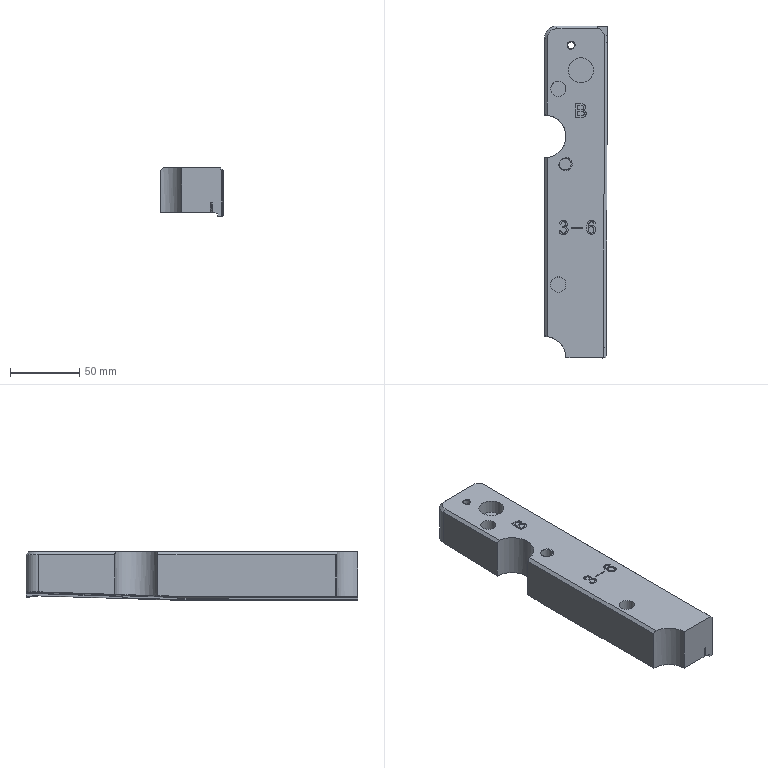NC program | NX | posted with a generic post | part box 45.476 x 239.737 x 35.001 mm
Lines 3829 to 4891 of 16758:
(CAVITY_MILL_2_COPY_COPY , TOOL : D16R0.8)
N7620 M6
N7622 G53
N7624 G17 G0 G90 X0.001 Y34.455 S2500 M3
N7626 G43 Z60. H0
N7628 G94 G1 Z35.502 F4000.
N7630 Z35.302 F1380.
N7632 Y23.255
N7634 X119.894 F2300.
N7636 G2 X120.382 Y22.789 R0.488
N7638 G1 X120.384 Y22.67
N7640 X120.387 Y-22.681
N7642 X120.385 Y-22.757
N7644 G2 X119.873 Y-23.255 R0.512
N7646 G1 X-119.865
N7648 G2 X-120.384 Y-22.735 R0.52
N7650 G1 X-120.383 Y22.748
N7652 G2 X-119.876 Y23.255 R0.507
N7654 G1 X0.001
N7656 Y13.895
N7658 X111.025
N7660 X111.027 Y-13.895
N7662 X-111.024
N7664 Y13.895
N7666 X0.001
N7668 Y4.535
N7670 X101.665
N7672 X101.666 Y-4.535
N7674 X-101.664
N7676 Y4.535
N7678 X0.001
N7680 Y15.735
N7682 Z35.502
N7684 G0 Z36.501
N7686 X0. Y34.626
N7688 G1 Z35.303 F4000.
N7690 Z35.103 F1380.
N7692 Y23.426
N7694 X119.382 F2300.
N7696 X120.095 Y23.387
N7698 G2 X120.557 Y22.846 R0.71
N7700 G1 X120.556 Y-22.731
N7702 G2 X119.86 Y-23.426 R0.695
N7704 G1 X-119.856
N7706 G2 X-120.557 Y-22.726 R0.7
N7708 G1 X-120.556 Y22.727
N7710 G2 X-119.857 Y23.426 R0.699
N7712 G1 X0.
N7714 Y14.066
N7716 X111.196
N7718 Y-14.066
N7720 X-111.197
N7722 X-111.196 Y14.066
N7724 X0.
N7726 Y4.706
N7728 X101.836
N7730 Y-4.706
N7732 X-101.836
N7734 Y4.706
N7736 X0.
N7738 Y15.906
N7740 Z35.303
N7742 G0 Z36.302
N7744 Y-34.698
N7746 G1 Z35.104 F4000.
N7748 Z34.904 F1380.
N7750 Y-23.498
N7752 X-119.893 F2300.
N7754 G2 X-120.628 Y-22.763 R0.735
N7756 G1 Y9.225
N7758 G2 X-127.828 Y13.401 R9.78
N7760 G1 Y22.763
N7762 G2 X-119.892 Y30.698 R7.935
N7764 G1 X18.758
N7766 G2 X24.095 Y23.498 R9.198
N7768 G1 X119.871
N7770 G2 X120.626 Y22.786 R0.757
N7772 G1 X120.628 Y22.753
N7774 Y-22.744
N7776 G2 X119.874 Y-23.498 R0.754
N7778 G1 X0.
N7780 Y-14.138
N7782 X-111.268
N7784 Y9.225
N7786 Y9.236
N7788 X-31.236 Y9.681
N7790 X-31.159 Y9.68
N7792 X-30.139 Y9.685
N7794 X-30.126
N7796 X10.322 Y10.191
N7798 G3 X10.94 Y10.218 R9.834
N7800 G1 X11.005 Y10.224
N7802 X15.047 Y10.672
N7804 X15.182 Y10.692
N7806 X16.595 Y10.954
N7808 G3 X22.188 Y14.334 R9.266
N7810 G1 X20.717 Y15.492
N7812 G2 X16.254 Y12.794 R7.394
N7814 G1 X14.841 Y12.532
N7816 X10.799 Y12.085
N7818 G2 X10.299 Y12.063 R7.962
N7820 G1 X-30.15 Y11.557
N7822 X-31.169 Y11.552
N7824 X-31.176 Y11.553
N7826 X-119.826 Y11.061
N7828 G2 X-127.695 Y19.051 R7.908
N7830 G1 Y21.655
N7832 G2 X-119.907 Y29.486 R7.877
N7834 G1 X-112.141 Y29.53
N7836 X10.126 Y30.106
N7838 G2 X16.365 Y29.507 R32.892
N7840 X22.3 Y22.314 R7.326
N7842 G1 Y20.064
N7844 G2 X20.717 Y15.492 R7.394
N7846 G1 X22.188 Y14.334
N7848 G3 X24.095 Y14.138 R9.36
N7850 G1 X111.268
N7852 Y-14.138
N7854 X0.
N7856 Y-4.778
N7858 X-101.908
N7860 Y-0.072
N7862 X-31.281 Y0.32
N7864 X-31.204 Y0.319
N7866 X-30.071 Y0.326
N7868 X-30.025
N7870 X10.439 Y0.832
N7872 G3 X11.727 Y0.891 R19.194
N7874 G1 X11.954 Y0.912
N7876 X16.077 Y1.369
N7878 G3 X16.888 Y1.489 R11.232
N7880 G1 X18.301 Y1.751
N7882 G3 X25.548 Y4.778 R18.626
N7884 G1 X101.908
N7886 Y-4.778
N7888 X0.
N7890 Y-15.978
N7892 Z35.104
N7894 G0 Z36.103
N7896 X65.496 Y-34.737
N7898 G1 Z34.905 F4000.
N7900 Z34.705 F1380.
N7902 Y-23.537
N7904 X-119.857 F2300.
N7906 G2 X-120.668 Y-22.726 R0.811
N7908 G1 Y8.941
N7910 G2 X-127.868 Y13.053 R10.045
N7912 G1 Y18.186
N7914 G3 X-119.825 Y10.769 R8.173
N7916 G1 X-31.237 Y11.262
N7918 X-31.168 Y11.261
N7920 X-30.174 Y11.267
N7922 X-30.119
N7924 X10.302 Y11.772
N7926 G3 X10.582 Y11.781 R8.253
N7928 G1 X15.201 Y12.084
N7930 X19.819 Y12.387
N7932 X22.493 Y12.825
N7934 G3 X28.719 Y20.152 R7.425
N7936 G1 Y22.331
N7938 G3 X21.74 Y29.771 R7.546
N7940 X10.158 Y30.313 R138.168
N7942 G1 X-112.142 Y29.737
N7944 X-112.172 Y29.733
N7946 X-119.866 Y29.692
N7948 G3 X-127.868 Y22.394 R8.04
N7950 G1 Y22.728
N7952 G2 X-119.859 Y30.737 R8.009
N7954 G1 X25.248
N7956 G2 X30.503 Y23.537 R9.418
N7958 G1 X119.858
N7960 G2 X120.668 Y22.728 R0.809
N7962 G1 Y-22.726
N7964 G2 X119.857 Y-23.537 R0.811
N7966 G1 X65.496
N7968 Y-14.177
N7970 X-111.308
N7972 Y1.457
N7974 X-31.245 Y1.901
N7976 X-31.176
N7978 X-30.106 Y1.907
N7980 X-30.019 Y1.908
N7982 X10.419 Y2.413
N7984 G3 X11.106 Y2.435 R17.613
N7986 G1 X20.884 Y3.077
N7988 X24.004 Y3.588
N7990 G3 X36.98 Y14.177 R16.785
N7992 G1 X111.308
N7994 Y-14.177
N7996 X65.496
N7998 Y-4.817
N8000 X29.045
N8002 X21.886 Y-4.053
N8004 G2 X21.356 Y-4.108 R7.2
N8006 G1 X11.578 Y-4.75
N8008 X11.474 Y-4.756
N8010 G2 X10.509 Y-4.786 R24.813
N8012 G1 X-29.929 Y-5.292
N8014 X-29.954
N8016 X-30.041 Y-5.293
N8018 X-30.066
N8020 X-31.136 Y-5.299
N8022 X-31.229
N8024 X-31.252
N8026 X-104.108 Y-5.703
N8028 Y-6.977
N8030 X22.177
N8032 G2 X21.886 Y-4.053 R7.2
N8034 G1 X29.045 Y-4.817
N8036 G3 X42.47 Y4.817 R26.145
N8038 G1 X101.948
N8040 Y-4.817
N8042 X65.496
N8044 Y-16.017
N8046 Z34.905
N8048 G0 Z35.904
N8050 X68.725 Y-34.738
N8052 G1 Z34.707 F4000.
N8054 Z34.507 F1380.
N8056 Y-23.538
N8058 X-119.857 F2300.
N8060 G2 X-120.668 Y-22.726 R0.811
N8062 G1 Y8.754
N8064 G2 X-127.868 Y12.772 R10.07
N8066 G1 Y17.387
N8068 G3 X-119.824 Y10.587 R8.198
N8070 G1 X-31.206 Y11.08
N8072 X-31.167 Y11.079
N8074 X-30.145 Y11.085
N8076 X9.799 Y11.584
N8078 X10.305 Y11.591
N8080 X10.307
N8082 X10.495 Y11.595
N8084 G3 X28.35 Y12.722 R243.063
N8086 X35.138 Y20.225 R7.54
N8088 G1 Y22.367
N8090 G3 X28.133 Y29.847 R7.496
N8092 X10.159 Y30.422 R268.337
N8094 G1 X-112.142 Y29.846
N8096 X-112.172 Y29.831
N8098 X-119.867 Y29.792
N8100 G3 X-127.849 Y23.271 R8.137
N8102 G2 X-119.855 Y30.737 R8.013
N8104 G1 X31.849
N8106 G2 X36.937 Y23.537 R9.368
N8108 G1 X119.858
N8110 G2 X120.668 Y22.728 R0.81
N8112 G1 Y-22.726
N8114 G2 X119.856 Y-23.538 R0.811
N8116 G1 X68.725
N8118 Y-14.178
N8120 X-111.308
N8122 Y1.275
N8124 X-31.225 Y1.72
N8126 X-31.187 Y1.719
N8128 X-30.061 Y1.725
N8130 X10.426 Y2.231
N8132 G3 X10.774 Y2.239 R17.795
N8134 X29.283 Y3.409 R252.423
N8136 X43.379 Y14.177 R16.9
N8138 G1 X111.308
N8140 Y-14.178
N8142 X68.725
N8144 Y-4.818
N8146 X35.503
N8148 X28.359 Y-3.914
N8150 G2 X10.984 Y-4.958 R259.623
N8152 X10.516 Y-4.968 R24.995
N8154 G1 X-29.971 Y-5.474
N8156 X-30.021
N8158 X-31.147 Y-5.481
N8160 X-31.238
N8162 X-104.108 Y-5.886
N8164 Y-6.978
N8166 X28.634
N8168 G2 X28.359 Y-3.914 R7.2
N8170 G1 X35.503 Y-4.818
N8172 G3 X48.863 Y4.817 R26.26
N8174 G1 X101.948
N8176 Y-4.818
N8178 X68.725
N8180 Y-16.018
N8182 Z34.707
N8184 G0 Z35.705
N8186 X71.638 Y-34.738
N8188 G1 Z34.508 F4000.
N8190 Z34.308 F1380.
N8192 Y-23.538
N8194 X-119.857 F2300.
N8196 G2 X-120.668 Y-22.726 R0.811
N8198 G1 Y8.627
N8200 G2 X-127.868 Y12.595 R10.071
N8202 G1 Y17.045
N8204 G3 X-119.824 Y10.464 R8.199
N8206 G1 X-31.206 Y10.956
N8208 X-31.167
N8210 X-30.144 Y10.962
N8212 X10.306 Y11.468
N8214 X10.434 Y11.47
N8216 X10.758 Y11.493
N8218 G3 X14.853 Y11.605 R512.62
N8220 X32.063 Y12.434 R512.62
N8222 X36.386 Y13.246 R18.276
N8224 X41.558 Y20.305 R7.404
N8226 G1 Y22.392
N8228 X38.802 Y28.145
N8230 G3 X34.912 Y29.739 R7.536
N8232 G1 X31.398 Y30.114
N8234 G3 X10.159 Y30.472 R579.431
N8236 G1 X-50.992 Y30.184
N8238 X-112.142 Y29.897
N8240 X-112.172 Y29.891
N8242 X-119.868 Y29.852
N8244 G3 X-127.814 Y23.651 R8.201
N8246 G2 X-119.855 Y30.737 R8.013
N8248 G1 X38.163
N8250 G2 X39.967 Y29.61 R9.408
N8252 X40.491 Y28.953 R1.872
N8254 G1 X43.084 Y23.537
N8256 X119.858
N8258 G2 X120.668 Y22.728 R0.81
N8260 G1 Y-22.726
N8262 G2 X119.856 Y-23.538 R0.811
N8264 G1 X71.638
N8266 Y-14.178
N8268 X-111.308
N8270 Y1.151
N8272 X-31.2 Y1.596
N8274 X-31.16
N8276 X11.196 Y2.141
N8278 G3 X15.146 Y2.249 R521.98
N8280 X32.67 Y3.094 R521.98
N8282 X39.207 Y4.321 R27.636
N8284 X49.758 Y14.177 R16.764
N8286 G1 X111.308
N8288 Y-14.178
N8290 X71.638
N8292 Y-4.818
N8294 X41.328
N8296 X34.174 Y-4.008
N8298 G2 X33.138 Y-4.091 R34.836
N8300 X15.371 Y-4.947 R529.18
N8302 X11.367 Y-5.057 R529.18
N8304 G1 X11.288 Y-5.059
N8306 X-31.068 Y-5.603
N8308 X-31.19 Y-5.604
N8310 X-31.195
N8312 X-104.108 Y-6.009
N8314 Y-6.978
N8316 X34.46
N8318 G2 X34.174 Y-4.008 R7.2
N8320 G1 X41.328 Y-4.818
N8322 G3 X42.029 Y-4.604 R36.996
N8324 X55.192 Y4.817 R26.124
N8326 G1 X101.948
N8328 Y-4.818
N8330 X71.638
N8332 Y-16.018
N8334 Z34.508
N8336 G0 Z35.507
N8338 X74.712 Y-34.738
N8340 G1 Z34.309 F4000.
N8342 Z34.109 F1380.
N8344 Y-23.538
N8346 X-119.857 F2300.
N8348 G2 X-120.668 Y-22.726 R0.811
N8350 G1 Y8.544
N8352 G2 X-127.868 Y12.486 R10.069
N8354 G1 Y16.865
N8356 G3 X-119.823 Y10.383 R8.197
N8358 G1 X-31.206 Y10.875
N8360 X-31.167
N8362 X-30.172 Y10.881
N8364 X-30.115
N8366 X-10.031 Y11.132
N8368 X10.307 Y11.386
N8370 X10.347 Y11.387
N8372 X10.386 Y11.388
N8374 G3 X37.61 Y12.442 R719.899
N8376 X42.479 Y13.224 R24.33
N8378 X47.977 Y20.38 R7.407
N8380 G1 Y22.432
N8382 Y22.433
N8384 G3 X41.723 Y29.697 R7.347
N8386 X35.459 Y30.25 R51.438
N8388 X13.134 Y30.493 R694.868
N8390 G1 X-112.17 Y29.903
N8392 X-112.175
N8394 X-119.913 Y29.862
N8396 G3 X-127.806 Y23.723 R8.2
N8398 G2 X-119.855 Y30.737 R8.013
N8400 G1 X44.63
N8402 G2 X49.782 Y23.537 R9.219
N8404 G1 X119.858
N8406 G2 X120.668 Y22.728 R0.81
N8408 G1 Y-22.726
N8410 G2 X119.856 Y-23.538 R0.811
N8412 G1 X74.712
N8414 Y-14.178
N8416 X-111.308
N8418 Y1.07
N8420 X-31.181 Y1.515
N8422 X-31.142
N8424 X-30.104 Y1.521
N8426 X-30.014 Y1.522
N8428 X10.579 Y2.03
N8430 G3 X38.149 Y3.097 R729.258
N8432 X44.892 Y4.18 R33.69
N8434 X56.148 Y14.177 R16.767
N8436 G1 X111.308
N8438 Y-14.178
N8440 X74.712
N8442 Y-4.818
N8444 X47.476
N8446 X40.329 Y-3.95
N8448 G2 X38.564 Y-4.091 R40.89
N8450 X10.721 Y-5.169 R736.458
N8452 G1 X10.669 Y-5.17
N8454 X-29.924 Y-5.678
N8456 X-29.949
N8458 X-30.039 Y-5.679
N8460 X-30.064
N8462 X-31.102 Y-5.685
N8464 X-31.144
N8466 X-31.162
N8468 X-104.108 Y-6.09
N8470 Y-6.978
N8472 X40.608
N8474 G2 X40.329 Y-3.95 R7.2
N8476 G1 X47.476 Y-4.818
N8478 G3 X61.556 Y4.817 R26.127
N8480 G1 X101.948
N8482 Y-4.818
N8484 X74.712
N8486 Y-16.018
N8488 Z34.309
N8490 G0 Z35.308
N8492 X77.911 Y-34.738
N8494 G1 Z34.11 F4000.
N8496 Z33.91 F1380.
N8498 Y-23.538
N8500 X-119.857 F2300.
N8502 G2 X-120.668 Y-22.726 R0.811
N8504 G1 Y8.496
N8506 G2 X-127.868 Y12.42 R10.079
N8508 G1 Y16.739
N8510 G3 X-119.823 Y10.335 R8.207
N8512 G1 X-31.206 Y10.828
N8514 X-31.167
N8516 X-30.171 Y10.833
N8518 X-30.115 Y10.834
N8520 X10.344 Y11.34
N8522 X18.783 Y11.511
N8524 G3 X46.539 Y12.74 R509.608
N8526 X54.396 Y20.455 R8.499
N8528 G1 Y22.468
N8530 G3 X48.156 Y29.719 R7.333
N8532 X41.334 Y30.31 R54.268
N8534 X19.553 Y30.523 R800.697
N8536 G1 X-112.17 Y29.903
N8538 X-112.175
N8540 X-119.913 Y29.862
N8542 X-119.931
N8544 G3 X-127.806 Y23.723 R8.2
N8546 G2 X-119.855 Y30.738 R8.013
N8548 G1 X51.106
N8550 G2 X56.206 Y23.538 R9.205
N8552 G1 X119.858
N8554 G2 X120.668 Y22.728 R0.81
N8556 G1 Y-22.73
N8558 G2 X119.86 Y-23.538 R0.807
N8560 G1 X77.911
N8562 Y-14.178
N8564 X-111.308
N8566 Y1.022
N8568 X-31.165 Y1.468
N8570 X-31.126
N8572 X-30.103 Y1.474
N8574 X-30.014
N8576 X10.497 Y1.981
N8578 X18.958 Y2.152
N8580 G3 X47.208 Y3.403 R518.968
N8582 X62.345 Y14.178 R17.859
N8584 G1 X111.308
N8586 Y-14.178
N8588 X77.911
N8590 Y-4.818
N8592 X53.874
N8594 X46.74 Y-3.848
N8596 G2 X19.092 Y-5.046 R526.168
N8598 G1 X10.643 Y-5.218
N8600 X10.587 Y-5.219
N8602 X-29.924 Y-5.725
N8604 X-29.949
N8606 X-30.038 Y-5.726
N8608 X-30.063
N8610 X-31.086 Y-5.732
N8612 X-31.103
N8614 X-31.133
N8616 X-104.108 Y-6.138
N8618 Y-6.978
N8620 X47.006
N8622 G2 X46.74 Y-3.848 R7.2
N8624 G1 X53.874 Y-4.818
N8626 G3 X67.656 Y4.818 R27.219
N8628 G1 X101.948
N8630 Y-4.818
N8632 X77.911
N8634 Y-16.018
N8636 Z34.11
N8638 G0 Z35.109
N8640 X81.127 Y-34.738
N8642 G1 Z33.911 F4000.
N8644 Z33.711 F1380.
N8646 Y-23.538
N8648 X-119.857 F2300.
N8650 G2 X-120.668 Y-22.726 R0.811
N8652 G1 Y8.478
N8654 G2 X-127.868 Y12.397 R10.08
N8656 G1 Y16.702
N8658 G3 X-119.823 Y10.318 R8.208
N8660 G1 X-112.117 Y10.361
N8662 X-112.074
N8664 X-30.171 Y10.816
N8666 X-30.114 Y10.817
N8668 X11.017 Y11.331
N8670 G3 X27.906 Y11.649 R1621.992
N8672 G1 X36.631 Y11.919
N8674 G3 X53.512 Y12.87 R334.668
N8676 X60.815 Y20.49 R7.957
N8678 G1 Y22.494
N8680 G3 X54.652 Y29.734 R7.335
N8682 X48.352 Y30.321 R46.943
N8684 X25.973 Y30.553 R741.905
N8686 G1 X-112.17 Y29.903
N8688 X-112.175
N8690 X-119.913 Y29.862
N8692 G3 X-127.806 Y23.723 R8.2
N8694 G2 X-119.855 Y30.738 R8.013
N8696 G1 X57.58
N8698 G2 X62.628 Y23.538 R9.207
N8700 G1 X119.858
N8702 G2 X120.668 Y22.728 R0.81
N8704 G1 Y-22.73
N8706 G2 X119.86 Y-23.538 R0.807
N8708 G1 X81.127
N8710 Y-14.178
N8712 X-111.308
N8714 Y1.006
N8716 X-30.103 Y1.457
N8718 X-30.014
N8720 X11.139 Y1.972
N8722 G3 X28.163 Y2.292 R1631.352
N8724 G1 X36.921 Y2.564
N8726 G3 X54.274 Y3.541 R344.028
N8728 X68.865 Y14.178 R17.317
N8730 G1 X111.308
N8732 Y-14.178
N8734 X81.127
N8736 Y-4.818
N8738 X60.307
N8740 X53.184 Y-3.768
N8742 G2 X37.145 Y-4.633 R351.228
N8744 G1 X28.386 Y-4.905
N8746 X28.336 Y-4.906
N8748 G2 X11.229 Y-5.228 R1638.552
N8750 G1 X-29.924 Y-5.742
N8752 X-29.949
N8754 X-30.038 Y-5.743
N8756 X-30.063
N8758 X-104.108 Y-6.155
N8760 Y-6.978
N8762 X53.439
N8764 G2 X53.184 Y-3.768 R7.2
N8766 G1 X60.307 Y-4.818
N8768 G3 X74.223 Y4.818 R26.677
N8770 G1 X101.948
N8772 Y-4.818
N8774 X81.127
N8776 Y-16.018
N8778 Z33.911
N8780 G0 Z34.91
N8782 X84.383 Y-34.738
N8784 G1 Z33.712 F4000.
N8786 Z33.512 F1380.
N8788 Y-23.538
N8790 X-119.857 F2300.
N8792 G2 X-120.668 Y-22.726 R0.811
N8794 G1 Y8.473
N8796 G2 X-127.868 Y12.392 R10.079
N8798 G1 Y16.697
N8800 G3 X-119.823 Y10.313 R8.207
N8802 G1 X-112.074 Y10.356
N8804 X-30.171 Y10.811
N8806 X-30.114 Y10.812
N8808 X17.436 Y11.406
N8810 G3 X39.481 Y11.873 R1308.21
N8812 G1 X40.467 Y11.908
N8814 X42.438 Y11.965
N8816 X56.237 Y12.59
N8818 X60.324 Y12.941
N8820 G3 X67.235 Y20.472 R7.558
N8822 G1 Y22.547
N8824 G3 X61.444 Y29.684 R7.293
N8826 X56.938 Y30.235 R26.497
N8828 X32.392 Y30.583 R563.158
N8830 G1 X-112.17 Y29.903
N8832 X-112.175
N8834 X-119.913 Y29.862
N8836 G3 X-127.806 Y23.723 R8.2
N8838 G2 X-119.855 Y30.738 R8.013
N8840 G1 X64.055
N8842 G2 X69.053 Y23.538 R9.165
N8844 G1 X119.858
N8846 G2 X120.668 Y22.728 R0.81
N8848 G1 Y-22.73
N8850 G2 X119.86 Y-23.538 R0.807
N8852 G1 X84.383
N8854 Y-14.178
N8856 X-111.308
N8858 Y1.
N8860 X-30.103 Y1.451
N8862 X-30.014 Y1.452
N8864 X17.555 Y2.047
N8866 G3 X39.787 Y2.518 R1317.57
N8868 G1 X40.769 Y2.553
N8870 X42.785 Y2.611
N8872 X56.85 Y3.248
N8874 X61.126 Y3.616
N8876 G3 X75.38 Y14.178 R16.918
N8878 G1 X111.308
N8880 Y-14.178
N8882 X84.383
N8884 Y-4.818
N8886 X66.818
N8888 X59.7 Y-3.733
N8890 X57.467 Y-3.925
N8892 G2 X57.176 Y-3.945 R7.2
N8894 G1 X43.11 Y-4.581
N8896 X42.992 Y-4.586
N8898 X41.001 Y-4.643
N8900 X40.045 Y-4.677
N8902 X40.001 Y-4.679
N8904 G2 X17.645 Y-5.153 R1324.77
N8906 G1 X-29.924 Y-5.747
N8908 X-29.949
N8910 X-30.038 Y-5.748
N8912 X-30.063
N8914 X-104.108 Y-6.16
N8916 Y-6.978
N8918 X59.949
N8920 G2 X59.7 Y-3.733 R7.2
N8922 G1 X66.818 Y-4.818
N8924 G3 X80.783 Y4.818 R26.278
N8926 G1 X101.948
N8928 Y-4.818
N8930 X84.383
N8932 Y-16.018
N8934 Z33.712
N8936 G0 Z34.711
N8938 X87.501 Y-34.738
N8940 G1 Z33.514 F4000.
N8942 Z33.314 F1380.
N8944 Y-23.538
N8946 X-119.857 F2300.
N8948 G2 X-120.668 Y-22.726 R0.811
N8950 G1 Y8.468
N8952 G2 X-127.868 Y12.387 R10.079
N8954 G1 Y16.693
N8956 G3 X-119.823 Y10.308 R8.207
N8958 G1 X-112.074 Y10.351
N8960 X-110.202 Y10.361
N8962 X-30.171 Y10.806
N8964 X-30.114 Y10.807
N8966 X22.726 Y11.467
N8968 G3 X50.295 Y12.093 R1258.898
N8970 G1 X50.323 Y12.098
N8972 X54.695 Y12.21
N8974 G3 X66.59 Y12.938 R167.491
N8976 X73.654 Y20.48 R7.823
N8978 G1 Y22.565
N8980 G3 X67.609 Y29.773 R7.321
N8982 G1 X66.093 Y30.041
N8984 X60.18 Y30.399
N8986 G3 X38.811 Y30.613 R651.504
N8988 G1 X-112.17 Y29.903
N8990 X-112.173
N8992 X-112.175
N8994 X-119.913 Y29.862
N8996 G3 X-127.806 Y23.723 R8.2
N8998 G2 X-119.855 Y30.738 R8.013
N9000 G1 X70.541
N9002 G2 X75.474 Y23.538 R9.193
N9004 G1 X119.858
N9006 G2 X120.668 Y22.728 R0.81
N9008 G1 Y-22.73
N9010 G2 X119.86 Y-23.538 R0.807
N9012 G1 X87.501
N9014 Y-14.178
N9016 X-111.308
N9018 Y0.995
N9020 X-30.014 Y1.447
N9022 X22.839 Y2.108
N9024 G3 X50.61 Y2.738 R1268.258
N9026 G1 X51.198 Y2.758
N9028 X54.934 Y2.853
N9030 G3 X67.494 Y3.622 R176.851
N9032 X81.722 Y14.178 R17.183
N9034 G1 X111.308
N9036 Y-14.178
N9038 X87.501
N9040 Y-4.818
N9042 X73.055
N9044 X65.935 Y-3.749
N9046 G2 X55.118 Y-4.344 R184.051
N9048 G1 X51.411 Y-4.439
N9050 X50.852 Y-4.458
N9052 G2 X22.929 Y-5.092 R1275.458
N9054 G1 X-29.924 Y-5.752
N9056 X-29.974 Y-5.753
N9058 X-104.108 Y-6.165
N9060 Y-6.978
N9062 X66.187
N9064 G2 X65.935 Y-3.749 R7.2
N9066 G1 X73.055 Y-4.818
N9068 G3 X87.083 Y4.818 R26.543
N9070 G1 X101.948
N9072 Y-4.818
N9074 X87.501
N9076 Y-16.018
N9078 Z33.514
N9080 G0 Z34.512
N9082 X90.701 Y-34.738
N9084 G1 Z33.315 F4000.
N9086 Z33.115 F1380.
N9088 Y-23.538
N9090 X-119.857 F2300.
N9092 G2 X-120.668 Y-22.726 R0.811
N9094 G1 Y8.463
N9096 G2 X-127.868 Y12.382 R10.079
N9098 G1 Y16.688
N9100 G3 X-119.823 Y10.303 R8.207
N9102 G1 X-112.074 Y10.346
N9104 X-110.202 Y10.356
N9106 X-30.171 Y10.801
N9108 X-30.114
N9110 X28.64 Y11.536
N9112 X36.525 Y11.649
N9114 G3 X60.442 Y12.182 R13074.106
N9116 X73.402 Y13.033 R153.378
N9118 X80.073 Y20.465 R7.476
N9120 G1 Y22.705
N9122 Y22.707
N9124 G3 X74.929 Y29.491 R7.047
N9126 X69.69 Y30.305 R22.258
N9128 X45.23 Y30.644 R585.99
N9130 G1 X-112.17 Y29.903
N9132 X-112.175
N9134 X-119.913 Y29.862
N9136 G3 X-127.806 Y23.723 R8.2
N9138 G2 X-119.855 Y30.738 R8.013
N9140 G1 X76.904
N9142 G2 X81.906 Y23.538 R8.919
N9144 G1 X119.858
N9146 G2 X120.668 Y22.728 R0.81
N9148 G1 Y-22.73
N9150 G2 X119.86 Y-23.538 R0.807
N9152 G1 X90.701
N9154 Y-14.178
N9156 X-111.308
N9158 Y0.99
N9160 X-30.014 Y1.442
N9162 X28.765 Y2.177
N9164 X36.692 Y2.29
N9166 G3 X60.659 Y2.824 R13083.466
N9168 X74.41 Y3.727 R162.738
N9170 X88.215 Y14.178 R16.836
N9172 G1 X111.308
N9174 Y-14.178
N9176 X90.701
N9178 Y-4.818
N9180 X79.454
N9182 X72.339 Y-3.715
N9184 G2 X60.826 Y-4.374 R169.938
N9186 X36.845 Y-4.908 R13090.667
N9188 G1 X36.795 Y-4.909
N9190 X28.868 Y-5.023
N9192 X28.855
N9194 X-29.924 Y-5.758
N9196 X-29.974
N9198 X-104.108 Y-6.17
N9200 Y-6.978
N9202 X72.586
N9204 G2 X72.339 Y-3.715 R7.2
N9206 G1 X79.454 Y-4.818
N9208 G3 X93.606 Y4.818 R26.196
N9210 G1 X101.948
N9212 Y-4.818
N9214 X90.701
N9216 Y-16.018
N9218 Z33.315
N9220 G0 Z34.314
N9222 X94.033 Y-34.738
N9224 G1 Z33.116 F4000.
N9226 Z32.916 F1380.
N9228 Y-23.538
N9230 X-119.857 F2300.
N9232 G2 X-120.668 Y-22.726 R0.811
N9234 G1 Y8.457
N9236 G2 X-127.868 Y12.377 R10.078
N9238 G1 Y16.683
N9240 G3 X-119.823 Y10.298 R8.206
N9242 G1 X-112.074 Y10.341
N9244 X-30.171 Y10.796
N9246 X-30.114
N9248 X-17.638 Y10.952
N9250 X10.89
N9252 X12.972 Y11.335
N9254 X35.539 Y11.617
N9256 X60.131 Y12.018
N9258 X65.108 Y12.136
N9260 G3 X79.594 Y12.932 R233.393
N9262 X86.492 Y20.451 R7.547
N9264 G1 Y22.71
N9266 G3 X81.39 Y29.51 R7.083
N9268 X76.083 Y30.357 R21.498
N9270 X51.65 Y30.674 R614.925
N9272 G1 X-112.17 Y29.903
N9274 X-112.175
N9276 X-119.913 Y29.862
N9278 G3 X-127.806 Y23.723 R8.2
N9280 G2 X-119.855 Y30.738 R8.013
N9282 G1 X83.378
N9284 G2 X88.326 Y23.538 R8.955
N9286 G1 X110.069
N9288 G2 X114.455 Y30.738 R9.695
N9290 G1 X119.858
N9292 G2 X127.868 Y22.728 R8.01
N9294 G1 Y15.306
N9296 G2 X120.668 Y10.916 R9.691
N9298 G1 Y-22.73
N9300 G2 X119.86 Y-23.538 R0.807
N9302 G1 X94.033
N9304 Y-14.178
N9306 X-111.308
N9308 Y0.985
N9310 X-30.103 Y1.436
N9312 X-30.014 Y1.437
N9314 X-17.58 Y1.592
N9316 X11.743
N9318 X13.883 Y1.985
N9320 X35.674 Y2.258
N9322 X60.319 Y2.66
N9324 X65.331 Y2.779
N9326 G3 X80.397 Y3.607 R242.753
N9328 X94.645 Y14.178 R16.907
N9330 G1 X110.069
N9332 G3 X111.97 Y14.373 R9.36
N9334 X111.308 Y10.916 R9.36
N9336 G1 Y-14.178
N9338 X94.033
N9340 Y-4.818
N9342 X86.118
N9344 X79. Y-3.732
N9346 G2 X65.502 Y-4.419 R249.953
N9348 G1 X60.49 Y-4.538
N9350 X60.436 Y-4.539
N9352 X35.791 Y-4.941
N9354 X35.764 Y-4.942
N9356 X14.584 Y-5.206
N9358 X13.045 Y-5.489
N9360 G2 X11.743 Y-5.608 R7.2
N9362 G1 X-17.535
N9364 X-29.924 Y-5.763
N9366 X-29.948
N9368 X-30.038 Y-5.764
N9370 X-30.063
N9372 X-104.108 Y-6.175
N9374 Y-6.978
N9376 X79.249
N9378 G2 X79. Y-3.732 R7.2
N9380 G1 X86.118 Y-4.818
N9382 G3 X100.053 Y4.818 R26.267
N9384 G1 X101.948
N9386 Y-4.818
N9388 X94.033
N9390 Y-16.018
N9392 Z33.116
N9394 G0 Z34.115
N9396 X118.575 Y41.584
N9398 G1 Z33.116 F4000.
N9400 Z32.916 F1380.
N9402 X119.248 Y30.405
N9404 G2 X127.49 Y23.488 R7.823 F2300.
N9406 G1 X127.521 Y23.22
N9408 X127.423 Y19.149
N9410 X127.347 Y18.816
N9412 G2 X111.907 Y20.514 R7.819
N9414 G1 X111.895 Y22.55
N9416 G2 X119.248 Y30.405 R7.823
N9418 G1 X118.575 Y41.584
N9420 Z33.116
N9422 G0 Z34.115
N9424 X97.154 Y-34.738
N9426 G1 Z32.917 F4000.
N9428 Z32.717 F1380.
N9430 Y-23.538
N9432 X-119.857 F2300.
N9434 G2 X-120.668 Y-22.726 R0.811
N9436 G1 Y7.994
N9438 G2 X-127.8 Y12.284 R9.5
N9440 G1 X-127.868 Y12.372
N9442 Y16.683
N9444 G3 X-126.274 Y13.372 R8.245
N9446 X-119.869 Y9.829 R7.628
N9448 G1 X-31.222
N9450 Y9.824
N9452 X10.89
N9454 X19.526 Y11.411
N9456 X43.113 Y11.706
N9458 X51.309 Y11.824
N9460 X52.295 Y11.83
N9462 G3 X74.818 Y12.221 R996.666
N9464 X85.992 Y12.956 R152.789
N9466 X92.911 Y20.464 R7.708
N9468 G1 Y22.737
N9470 G3 X87.882 Y29.522 R7.092
N9472 X82.771 Y30.37 R19.867
N9474 X58.069 Y30.704 R613.11
N9476 G1 X-112.17 Y29.903
N9478 X-112.175
N9480 X-119.913 Y29.862
N9482 G3 X-127.806 Y23.723 R8.2
N9484 G2 X-119.855 Y30.738 R8.013
N9486 G1 X89.863
N9488 G2 X94.748 Y23.538 R8.964
N9490 G1 X108.351
N9492 X108.353 Y23.546
N9494 G2 X113.008 Y30.738 R10.508
N9496 G1 X119.858
N9498 G2 X127.868 Y22.728 R8.01
N9500 G1 Y22.005
N9502 G3 X127.691 Y24.205 R19.303
N9504 X118.048 Y30.536 R8.06
N9506 X110.197 Y23.22 R8.636
N9508 X118.332 Y12.475 R8.995
N9510 X127.721 Y19.146 R7.976
N9512 X127.868 Y21.123 R19.303
N9514 G1 Y14.619
N9516 G2 X120.668 Y10.497 R9.848
N9518 G1 Y-22.73
N9520 G2 X119.86 Y-23.538 R0.807
N9522 G1 X97.154
N9524 Y-14.178
N9526 X-111.308
N9528 Y0.469
N9530 X-31.517
N9532 G3 X-31.222 Y0.464 R9.36
N9534 G1 X11.743
N9536 X20.437 Y2.062
N9538 X43.239 Y2.347
N9540 X51.402 Y2.465
N9542 G3 X75.086 Y2.865 R1006.026
N9544 X86.948 Y3.645 R162.149
N9546 X101.009 Y14.178 R17.068
N9548 G1 X102.159
N9550 G3 X111.308 Y4.785 R18.355
N9552 G1 Y-14.178
N9554 X97.154
N9556 Y-4.818
N9558 X92.36
N9560 X85.239 Y-3.751
N9562 G2 X75.293 Y-4.332 R169.349
N9564 X51.472 Y-4.735 R1013.226
N9566 G1 X43.342 Y-4.852
N9568 X43.329
N9570 X21.137 Y-5.13
N9572 X13.045 Y-6.617
N9574 G2 X11.743 Y-6.736 R7.2
N9576 G1 X-31.222
N9578 G2 X-31.615 Y-6.731 R16.56
N9580 G1 X-104.108
N9582 Y-6.978
N9584 X85.492
N9586 G2 X85.239 Y-3.751 R7.2
N9588 G1 X92.36 Y-4.818
N9590 G3 X101.592 Y-0.11 R26.428
N9592 X101.948 Y-0.393 R27.715
N9594 G1 Y-4.818
N9596 X97.154
N9598 Y-16.018
N9600 Z32.917
N9602 G0 Z33.916
N9604 X100.467 Y-34.738
N9606 G1 Z32.718 F4000.
N9608 Z32.518 F1380.
N9610 Y-23.538
N9612 X-119.857 F2300.
N9614 G2 X-120.668 Y-22.726 R0.811
N9616 G1 Y6.869
N9618 G2 X-127.868 Y11.246 R9.59
N9620 G1 Y16.689
N9622 G3 X-127.529 Y15.342 R12.625
N9624 G1 X-127.23 Y14.357
N9626 G3 X-119.869 Y8.701 R7.718
N9628 G1 X-31.222
N9630 Y8.697
N9632 X10.89
N9634 X26.079 Y11.488
N9636 X50.395 Y11.792
N9638 X50.455
N9640 G3 X77.345 Y12.099 R1215.457
N9642 X92.418 Y12.92 R236.88
N9644 X99.331 Y20.455 R7.564
N9646 G1 Y22.764
N9648 G3 X94.369 Y29.535 R7.101
N9650 X89.449 Y30.382 R18.464
N9652 X71.945 Y30.738 R601.567
N9654 G1 X96.345
N9656 G2 X101.169 Y23.538 R8.973
N9658 G1 X106.642
N9660 G2 X108.346 Y28.144 R12.411
N9662 X110.911 Y30.738 R8.126
N9664 G1 X118.035
N9666 G3 X113.524 Y29.881 R24.62
N9668 X109.938 Y27.16 R6.254
N9670 X110.071 Y15.87 R10.539
N9672 X114.389 Y12.994 R8.215
N9674 X118.332 Y12.247 R20.668
N9676 X127.868 Y19.102 R8.147
N9678 G1 Y14.314
N9680 G2 X120.668 Y10.278 R10.019
N9682 G1 Y-22.73
N9684 G2 X119.86 Y-23.538 R0.807
N9686 G1 X100.467
N9688 Y-14.178
N9690 X-111.308
N9692 Y-0.659
N9694 X-31.517
N9696 G3 X-31.222 Y-0.663 R9.36
N9698 G1 X11.743
N9700 X26.99 Y2.139
N9702 X50.455 Y2.432
N9704 G3 X77.555 Y2.742 R1224.817
N9706 X93.224 Y3.594 R246.24
N9708 X103.931 Y8.688 R16.924
N9710 X111.308 Y4.145 R17.575
N9712 G1 Y-14.178
N9714 X100.467
N9716 Y-4.818
N9718 X98.987
N9720 X91.867 Y-3.742
N9722 G2 X77.717 Y-4.456 R253.44
N9724 X50.501 Y-4.768 R1232.017
N9726 G1 X27.691 Y-5.053
N9728 X17.219 Y-6.978
N9730 X92.118
N9732 G2 X91.867 Y-3.742 R7.2
N9734 G1 X98.987 Y-4.818
N9736 G3 X101.948 Y-3.777 R26.284
N9738 G1 Y-4.818